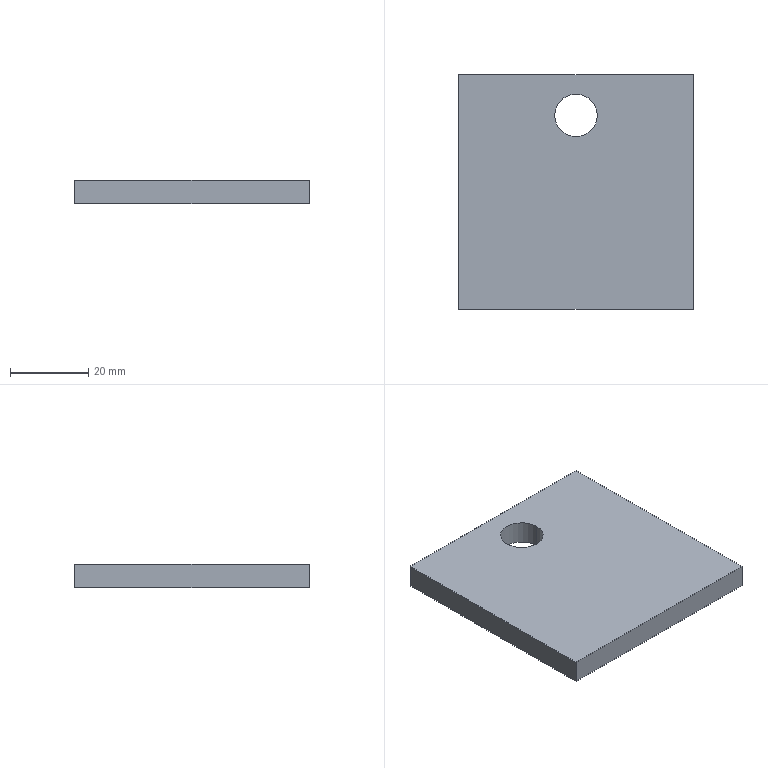Part | NX | features 凸台-拉伸21[6] 2 | 1 solid | 8 faces | box 60 x 60 x 6 mm | volume 21040 mm3 | plane 6 | cylinder 2 | commonest cylinder face diameters 10.905 x2
STEP:
#1=CARTESIAN_POINT('',(3517.548,-550.427,-1108.985));
#2=VERTEX_POINT('',#1);
#3=CARTESIAN_POINT('',(3517.548,-550.427,-1102.985));
#4=VERTEX_POINT('',#3);
#5=CARTESIAN_POINT('',(3517.548,-550.427,-1108.985));
#6=DIRECTION('',(0.,0.,1.));
#7=VECTOR('',#6,1000.);
#8=LINE('',#5,#7);
#9=EDGE_CURVE('',#2,#4,#8,.T.);
#10=ORIENTED_EDGE('',*,*,#9,.F.);
#11=CARTESIAN_POINT('',(3528.452,-550.427,-1108.985));
#12=VERTEX_POINT('',#11);
#13=CARTESIAN_POINT('',(3523.,-550.427,-1108.985));
#14=DIRECTION('',(0.,0.,-1.));
#15=DIRECTION('',(-1.,0.,0.));
#16=AXIS2_PLACEMENT_3D('',#13,#14,#15);
#17=CIRCLE('',#16,5.452);
#18=EDGE_CURVE('',#2,#12,#17,.T.);
#19=ORIENTED_EDGE('',*,*,#18,.T.);
#20=CARTESIAN_POINT('',(3528.452,-550.427,-1102.985));
#21=VERTEX_POINT('',#20);
#22=CARTESIAN_POINT('',(3528.452,-550.427,-1108.985));
#23=DIRECTION('',(0.,0.,1.));
#24=VECTOR('',#23,1000.);
#25=LINE('',#22,#24);
#26=EDGE_CURVE('',#21,#12,#25,.F.);
#27=ORIENTED_EDGE('',*,*,#26,.F.);
#28=CARTESIAN_POINT('',(3523.,-550.427,-1102.985));
#29=DIRECTION('',(0.,0.,-1.));
#30=DIRECTION('',(-1.,0.,0.));
#31=AXIS2_PLACEMENT_3D('',#28,#29,#30);
#32=CIRCLE('',#31,5.452);
#33=EDGE_CURVE('',#4,#21,#32,.T.);
#34=ORIENTED_EDGE('',*,*,#33,.F.);
#35=EDGE_LOOP('',(#10,#19,#27,#34));
#36=FACE_BOUND('',#35,.T.);
#37=CARTESIAN_POINT('',(3523.,-550.427,-1108.985));
#38=DIRECTION('',(0.,0.,1.));
#39=DIRECTION('',(1.,0.,0.));
#40=AXIS2_PLACEMENT_3D('',#37,#38,#39);
#41=CYLINDRICAL_SURFACE('',#40,5.452);
#42=ADVANCED_FACE('',(#36),#41,.F.);
#43=CARTESIAN_POINT('',(3493.,-540.,-1102.985));
#44=VERTEX_POINT('',#43);
#45=CARTESIAN_POINT('',(3553.,-540.,-1102.985));
#46=VERTEX_POINT('',#45);
#47=CARTESIAN_POINT('',(3553.,-540.,-1102.985));
#48=DIRECTION('',(1.,0.,0.));
#49=VECTOR('',#48,1000.);
#50=LINE('',#47,#49);
#51=EDGE_CURVE('',#44,#46,#50,.T.);
#52=ORIENTED_EDGE('',*,*,#51,.T.);
#53=CARTESIAN_POINT('',(3553.,-540.,-1108.985));
#54=VERTEX_POINT('',#53);
#55=CARTESIAN_POINT('',(3553.,-540.,-1108.985));
#56=DIRECTION('',(0.,0.,1.));
#57=VECTOR('',#56,1000.);
#58=LINE('',#55,#57);
#59=EDGE_CURVE('',#54,#46,#58,.T.);
#60=ORIENTED_EDGE('',*,*,#59,.F.);
#61=CARTESIAN_POINT('',(3493.,-540.,-1108.985));
#62=VERTEX_POINT('',#61);
#63=CARTESIAN_POINT('',(3553.,-540.,-1108.985));
#64=DIRECTION('',(1.,0.,0.));
#65=VECTOR('',#64,1000.);
#66=LINE('',#63,#65);
#67=EDGE_CURVE('',#62,#54,#66,.T.);
#68=ORIENTED_EDGE('',*,*,#67,.F.);
#69=CARTESIAN_POINT('',(3493.,-540.,-1108.985));
#70=DIRECTION('',(0.,0.,1.));
#71=VECTOR('',#70,1000.);
#72=LINE('',#69,#71);
#73=EDGE_CURVE('',#62,#44,#72,.T.);
#74=ORIENTED_EDGE('',*,*,#73,.T.);
#75=EDGE_LOOP('',(#52,#60,#68,#74));
#76=FACE_BOUND('',#75,.T.);
#77=CARTESIAN_POINT('',(3553.,-540.,-1108.985));
#78=DIRECTION('',(0.,-1.,0.));
#79=DIRECTION('',(0.,0.,-1.));
#80=AXIS2_PLACEMENT_3D('',#77,#78,#79);
#81=PLANE('',#80);
#82=ADVANCED_FACE('',(#76),#81,.F.);
#83=CARTESIAN_POINT('',(3493.,-600.,-1102.985));
#84=VERTEX_POINT('',#83);
#85=CARTESIAN_POINT('',(3493.,-600.,-1102.985));
#86=DIRECTION('',(0.,1.,0.));
#87=VECTOR('',#86,1000.);
#88=LINE('',#85,#87);
#89=EDGE_CURVE('',#84,#44,#88,.T.);
#90=ORIENTED_EDGE('',*,*,#89,.T.);
#91=ORIENTED_EDGE('',*,*,#73,.F.);
#92=CARTESIAN_POINT('',(3493.,-600.,-1108.985));
#93=VERTEX_POINT('',#92);
#94=CARTESIAN_POINT('',(3493.,-600.,-1108.985));
#95=DIRECTION('',(0.,1.,0.));
#96=VECTOR('',#95,1000.);
#97=LINE('',#94,#96);
#98=EDGE_CURVE('',#93,#62,#97,.T.);
#99=ORIENTED_EDGE('',*,*,#98,.F.);
#100=CARTESIAN_POINT('',(3493.,-600.,-1108.985));
#101=DIRECTION('',(0.,0.,1.));
#102=VECTOR('',#101,1000.);
#103=LINE('',#100,#102);
#104=EDGE_CURVE('',#93,#84,#103,.T.);
#105=ORIENTED_EDGE('',*,*,#104,.T.);
#106=EDGE_LOOP('',(#90,#91,#99,#105));
#107=FACE_BOUND('',#106,.T.);
#108=CARTESIAN_POINT('',(3493.,-600.,-1108.985));
#109=DIRECTION('',(1.,0.,0.));
#110=DIRECTION('',(0.,0.,-1.));
#111=AXIS2_PLACEMENT_3D('',#108,#109,#110);
#112=PLANE('',#111);
#113=ADVANCED_FACE('',(#107),#112,.F.);
#114=CARTESIAN_POINT('',(3553.,-600.,-1102.985));
#115=VERTEX_POINT('',#114);
#116=CARTESIAN_POINT('',(3553.,-600.,-1102.985));
#117=DIRECTION('',(-1.,0.,0.));
#118=VECTOR('',#117,1000.);
#119=LINE('',#116,#118);
#120=EDGE_CURVE('',#115,#84,#119,.T.);
#121=ORIENTED_EDGE('',*,*,#120,.T.);
#122=ORIENTED_EDGE('',*,*,#104,.F.);
#123=CARTESIAN_POINT('',(3553.,-600.,-1108.985));
#124=VERTEX_POINT('',#123);
#125=CARTESIAN_POINT('',(3553.,-600.,-1108.985));
#126=DIRECTION('',(-1.,0.,0.));
#127=VECTOR('',#126,1000.);
#128=LINE('',#125,#127);
#129=EDGE_CURVE('',#124,#93,#128,.T.);
#130=ORIENTED_EDGE('',*,*,#129,.F.);
#131=CARTESIAN_POINT('',(3553.,-600.,-1108.985));
#132=DIRECTION('',(0.,0.,1.));
#133=VECTOR('',#132,1000.);
#134=LINE('',#131,#133);
#135=EDGE_CURVE('',#124,#115,#134,.T.);
#136=ORIENTED_EDGE('',*,*,#135,.T.);
#137=EDGE_LOOP('',(#121,#122,#130,#136));
#138=FACE_BOUND('',#137,.T.);
#139=CARTESIAN_POINT('',(3553.,-600.,-1108.985));
#140=DIRECTION('',(0.,1.,0.));
#141=DIRECTION('',(0.,0.,1.));
#142=AXIS2_PLACEMENT_3D('',#139,#140,#141);
#143=PLANE('',#142);
#144=ADVANCED_FACE('',(#138),#143,.F.);
#145=CARTESIAN_POINT('',(3553.,-600.,-1102.985));
#146=DIRECTION('',(0.,-1.,0.));
#147=VECTOR('',#146,1000.);
#148=LINE('',#145,#147);
#149=EDGE_CURVE('',#46,#115,#148,.T.);
#150=ORIENTED_EDGE('',*,*,#149,.T.);
#151=ORIENTED_EDGE('',*,*,#135,.F.);
#152=CARTESIAN_POINT('',(3553.,-600.,-1108.985));
#153=DIRECTION('',(0.,-1.,0.));
#154=VECTOR('',#153,1000.);
#155=LINE('',#152,#154);
#156=EDGE_CURVE('',#54,#124,#155,.T.);
#157=ORIENTED_EDGE('',*,*,#156,.F.);
#158=ORIENTED_EDGE('',*,*,#59,.T.);
#159=EDGE_LOOP('',(#150,#151,#157,#158));
#160=FACE_BOUND('',#159,.T.);
#161=CARTESIAN_POINT('',(3553.,-600.,-1108.985));
#162=DIRECTION('',(-1.,0.,0.));
#163=DIRECTION('',(0.,0.,1.));
#164=AXIS2_PLACEMENT_3D('',#161,#162,#163);
#165=PLANE('',#164);
#166=ADVANCED_FACE('',(#160),#165,.F.);
#167=CARTESIAN_POINT('',(3523.,-550.427,-1102.985));
#168=DIRECTION('',(0.,0.,-1.));
#169=DIRECTION('',(-1.,0.,0.));
#170=AXIS2_PLACEMENT_3D('',#167,#168,#169);
#171=CIRCLE('',#170,5.452);
#172=EDGE_CURVE('',#21,#4,#171,.T.);
#173=ORIENTED_EDGE('',*,*,#172,.T.);
#174=ORIENTED_EDGE('',*,*,#33,.T.);
#175=EDGE_LOOP('',(#173,#174));
#176=FACE_BOUND('',#175,.T.);
#177=ORIENTED_EDGE('',*,*,#149,.F.);
#178=ORIENTED_EDGE('',*,*,#51,.F.);
#179=ORIENTED_EDGE('',*,*,#89,.F.);
#180=ORIENTED_EDGE('',*,*,#120,.F.);
#181=EDGE_LOOP('',(#177,#178,#179,#180));
#182=FACE_BOUND('',#181,.T.);
#183=CARTESIAN_POINT('',(3000.,0.,-1102.985));
#184=DIRECTION('',(0.,0.,1.));
#185=DIRECTION('',(1.,0.,0.));
#186=AXIS2_PLACEMENT_3D('',#183,#184,#185);
#187=PLANE('',#186);
#188=ADVANCED_FACE('',(#176,#182),#187,.T.);
#189=CARTESIAN_POINT('',(3523.,-550.427,-1108.985));
#190=DIRECTION('',(0.,0.,-1.));
#191=DIRECTION('',(-1.,0.,0.));
#192=AXIS2_PLACEMENT_3D('',#189,#190,#191);
#193=CIRCLE('',#192,5.452);
#194=EDGE_CURVE('',#12,#2,#193,.T.);
#195=ORIENTED_EDGE('',*,*,#194,.F.);
#196=ORIENTED_EDGE('',*,*,#18,.F.);
#197=EDGE_LOOP('',(#195,#196));
#198=FACE_BOUND('',#197,.T.);
#199=ORIENTED_EDGE('',*,*,#156,.T.);
#200=ORIENTED_EDGE('',*,*,#129,.T.);
#201=ORIENTED_EDGE('',*,*,#98,.T.);
#202=ORIENTED_EDGE('',*,*,#67,.T.);
#203=EDGE_LOOP('',(#199,#200,#201,#202));
#204=FACE_BOUND('',#203,.T.);
#205=CARTESIAN_POINT('',(3000.,0.,-1108.985));
#206=DIRECTION('',(0.,0.,1.));
#207=DIRECTION('',(1.,0.,0.));
#208=AXIS2_PLACEMENT_3D('',#205,#206,#207);
#209=PLANE('',#208);
#210=ADVANCED_FACE('',(#198,#204),#209,.F.);
#211=ORIENTED_EDGE('',*,*,#194,.T.);
#212=ORIENTED_EDGE('',*,*,#9,.T.);
#213=ORIENTED_EDGE('',*,*,#172,.F.);
#214=ORIENTED_EDGE('',*,*,#26,.T.);
#215=EDGE_LOOP('',(#211,#212,#213,#214));
#216=FACE_BOUND('',#215,.T.);
#217=CARTESIAN_POINT('',(3523.,-550.427,-1108.985));
#218=DIRECTION('',(0.,0.,1.));
#219=DIRECTION('',(1.,0.,0.));
#220=AXIS2_PLACEMENT_3D('',#217,#218,#219);
#221=CYLINDRICAL_SURFACE('',#220,5.452);
#222=ADVANCED_FACE('',(#216),#221,.F.);
#223=CLOSED_SHELL('',(#42,#82,#113,#144,#166,#188,#210,#222));
#224=MANIFOLD_SOLID_BREP('',#223);
#225=(LENGTH_UNIT()NAMED_UNIT(*)SI_UNIT(.MILLI.,.METRE.));
#226=UNCERTAINTY_MEASURE_WITH_UNIT(LENGTH_MEASURE(0.00001),#225,'','');
#227=(NAMED_UNIT(*)PLANE_ANGLE_UNIT()SI_UNIT($,.RADIAN.));
#228=(NAMED_UNIT(*)SI_UNIT($,.STERADIAN.)SOLID_ANGLE_UNIT());
#229=(GEOMETRIC_REPRESENTATION_CONTEXT(3)GLOBAL_UNCERTAINTY_ASSIGNED_CONTEXT((#226))GLOBAL_UNIT_ASSIGNED_CONTEXT((#225,#227,#228))REPRESENTATION_CONTEXT('',''));
#230=ADVANCED_BREP_SHAPE_REPRESENTATION('',(#224),#229);